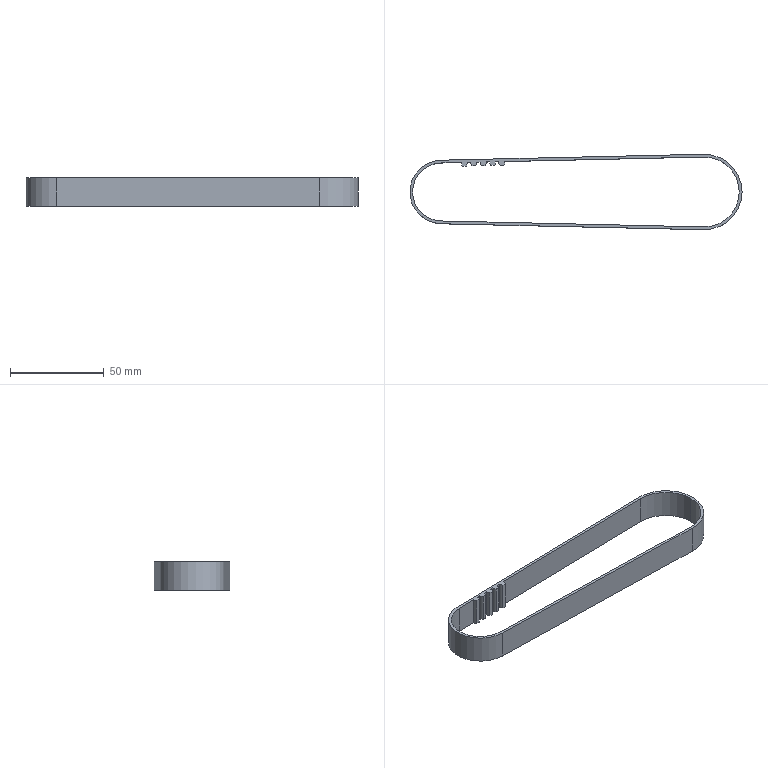Part | SolidWorks | features BaseBody 1 | 1 solid | 37 faces | box 177.014 x 40.237 x 15 mm | volume 9222 mm3 | cylinder 21 | plane 16 | commonest cylinder face diameters 6.5 x15 37.237 x2 40.237 x2 30.871 x1 33.871 x1
STEP:
#1=CARTESIAN_POINT('',(139.502,-20.113,-7.5));
#2=VERTEX_POINT('',#1);
#3=CARTESIAN_POINT('',(160.079,0.,-7.5));
#4=VERTEX_POINT('',#3);
#5=CARTESIAN_POINT('',(139.96,0.,-7.5));
#6=DIRECTION('',(0.,0.,1.));
#7=DIRECTION('',(1.,0.,0.));
#8=AXIS2_PLACEMENT_3D('',#5,#6,#7);
#9=CIRCLE('',#8,20.119);
#10=EDGE_CURVE('',#2,#4,#9,.T.);
#11=ORIENTED_EDGE('',*,*,#10,.T.);
#12=CARTESIAN_POINT('',(160.079,0.,7.5));
#13=VERTEX_POINT('',#12);
#14=CARTESIAN_POINT('',(160.079,0.,7.5));
#15=DIRECTION('',(0.,0.,1.));
#16=VECTOR('',#15,1000.);
#17=LINE('',#14,#16);
#18=EDGE_CURVE('',#4,#13,#17,.T.);
#19=ORIENTED_EDGE('',*,*,#18,.T.);
#20=CARTESIAN_POINT('',(139.502,-20.113,7.5));
#21=VERTEX_POINT('',#20);
#22=CARTESIAN_POINT('',(139.96,0.,7.5));
#23=DIRECTION('',(0.,0.,-1.));
#24=DIRECTION('',(1.,0.,0.));
#25=AXIS2_PLACEMENT_3D('',#22,#23,#24);
#26=CIRCLE('',#25,20.119);
#27=EDGE_CURVE('',#13,#21,#26,.T.);
#28=ORIENTED_EDGE('',*,*,#27,.T.);
#29=CARTESIAN_POINT('',(139.502,-20.113,7.5));
#30=DIRECTION('',(0.,0.,-1.));
#31=VECTOR('',#30,1000.);
#32=LINE('',#29,#31);
#33=EDGE_CURVE('',#21,#2,#32,.T.);
#34=ORIENTED_EDGE('',*,*,#33,.T.);
#35=EDGE_LOOP('',(#11,#19,#28,#34));
#36=FACE_OUTER_BOUND('',#35,.T.);
#37=CARTESIAN_POINT('',(139.96,0.,7.5));
#38=DIRECTION('',(0.,0.,1.));
#39=DIRECTION('',(1.,0.,0.));
#40=AXIS2_PLACEMENT_3D('',#37,#38,#39);
#41=CYLINDRICAL_SURFACE('',#40,20.119);
#42=ADVANCED_FACE('',(#36),#41,.T.);
#43=CARTESIAN_POINT('',(33.188,14.284,-7.5));
#44=VERTEX_POINT('',#43);
#45=CARTESIAN_POINT('',(33.766,16.134,-7.5));
#46=VERTEX_POINT('',#45);
#47=CARTESIAN_POINT('',(30.516,16.134,-7.5));
#48=DIRECTION('',(0.,0.,1.));
#49=DIRECTION('',(1.,0.,0.));
#50=AXIS2_PLACEMENT_3D('',#47,#48,#49);
#51=CIRCLE('',#50,3.25);
#52=EDGE_CURVE('',#44,#46,#51,.T.);
#53=ORIENTED_EDGE('',*,*,#52,.T.);
#54=CARTESIAN_POINT('',(33.766,16.134,7.5));
#55=VERTEX_POINT('',#54);
#56=CARTESIAN_POINT('',(33.766,16.134,7.5));
#57=DIRECTION('',(0.,0.,1.));
#58=VECTOR('',#57,1000.);
#59=LINE('',#56,#58);
#60=EDGE_CURVE('',#46,#55,#59,.T.);
#61=ORIENTED_EDGE('',*,*,#60,.T.);
#62=CARTESIAN_POINT('',(33.188,14.284,7.5));
#63=VERTEX_POINT('',#62);
#64=CARTESIAN_POINT('',(30.516,16.134,7.5));
#65=DIRECTION('',(0.,0.,1.));
#66=DIRECTION('',(1.,0.,0.));
#67=AXIS2_PLACEMENT_3D('',#64,#65,#66);
#68=CIRCLE('',#67,3.25);
#69=EDGE_CURVE('',#63,#55,#68,.T.);
#70=ORIENTED_EDGE('',*,*,#69,.F.);
#71=CARTESIAN_POINT('',(33.188,14.284,7.5));
#72=DIRECTION('',(0.,0.,-1.));
#73=VECTOR('',#72,1000.);
#74=LINE('',#71,#73);
#75=EDGE_CURVE('',#63,#44,#74,.T.);
#76=ORIENTED_EDGE('',*,*,#75,.T.);
#77=EDGE_LOOP('',(#53,#61,#70,#76));
#78=FACE_OUTER_BOUND('',#77,.T.);
#79=CARTESIAN_POINT('',(30.516,16.134,7.5));
#80=DIRECTION('',(0.,0.,1.));
#81=DIRECTION('',(1.,0.,0.));
#82=AXIS2_PLACEMENT_3D('',#79,#80,#81);
#83=CYLINDRICAL_SURFACE('',#82,3.25);
#84=ADVANCED_FACE('',(#78),#83,.T.);
#85=CARTESIAN_POINT('',(28.19,14.17,-7.5));
#86=VERTEX_POINT('',#85);
#87=CARTESIAN_POINT('',(28.767,16.02,-7.5));
#88=VERTEX_POINT('',#87);
#89=CARTESIAN_POINT('',(25.517,16.02,-7.5));
#90=DIRECTION('',(0.,0.,1.));
#91=DIRECTION('',(1.,0.,0.));
#92=AXIS2_PLACEMENT_3D('',#89,#90,#91);
#93=CIRCLE('',#92,3.25);
#94=EDGE_CURVE('',#86,#88,#93,.T.);
#95=ORIENTED_EDGE('',*,*,#94,.T.);
#96=CARTESIAN_POINT('',(28.767,16.02,7.5));
#97=VERTEX_POINT('',#96);
#98=CARTESIAN_POINT('',(28.767,16.02,7.5));
#99=DIRECTION('',(0.,0.,1.));
#100=VECTOR('',#99,1000.);
#101=LINE('',#98,#100);
#102=EDGE_CURVE('',#88,#97,#101,.T.);
#103=ORIENTED_EDGE('',*,*,#102,.T.);
#104=CARTESIAN_POINT('',(28.19,14.17,7.5));
#105=VERTEX_POINT('',#104);
#106=CARTESIAN_POINT('',(25.517,16.02,7.5));
#107=DIRECTION('',(0.,0.,1.));
#108=DIRECTION('',(1.,0.,0.));
#109=AXIS2_PLACEMENT_3D('',#106,#107,#108);
#110=CIRCLE('',#109,3.25);
#111=EDGE_CURVE('',#105,#97,#110,.T.);
#112=ORIENTED_EDGE('',*,*,#111,.F.);
#113=CARTESIAN_POINT('',(28.19,14.17,7.5));
#114=DIRECTION('',(0.,0.,-1.));
#115=VECTOR('',#114,1000.);
#116=LINE('',#113,#115);
#117=EDGE_CURVE('',#105,#86,#116,.T.);
#118=ORIENTED_EDGE('',*,*,#117,.T.);
#119=EDGE_LOOP('',(#95,#103,#112,#118));
#120=FACE_OUTER_BOUND('',#119,.T.);
#121=CARTESIAN_POINT('',(25.517,16.02,7.5));
#122=DIRECTION('',(0.,0.,1.));
#123=DIRECTION('',(1.,0.,0.));
#124=AXIS2_PLACEMENT_3D('',#121,#122,#123);
#125=CYLINDRICAL_SURFACE('',#124,3.25);
#126=ADVANCED_FACE('',(#120),#125,.T.);
#127=CARTESIAN_POINT('',(23.191,14.057,-7.5));
#128=VERTEX_POINT('',#127);
#129=CARTESIAN_POINT('',(23.769,15.906,-7.5));
#130=VERTEX_POINT('',#129);
#131=CARTESIAN_POINT('',(20.519,15.906,-7.5));
#132=DIRECTION('',(0.,0.,1.));
#133=DIRECTION('',(1.,0.,0.));
#134=AXIS2_PLACEMENT_3D('',#131,#132,#133);
#135=CIRCLE('',#134,3.25);
#136=EDGE_CURVE('',#128,#130,#135,.T.);
#137=ORIENTED_EDGE('',*,*,#136,.T.);
#138=CARTESIAN_POINT('',(23.769,15.906,7.5));
#139=VERTEX_POINT('',#138);
#140=CARTESIAN_POINT('',(23.769,15.906,7.5));
#141=DIRECTION('',(0.,0.,1.));
#142=VECTOR('',#141,1000.);
#143=LINE('',#140,#142);
#144=EDGE_CURVE('',#130,#139,#143,.T.);
#145=ORIENTED_EDGE('',*,*,#144,.T.);
#146=CARTESIAN_POINT('',(23.191,14.057,7.5));
#147=VERTEX_POINT('',#146);
#148=CARTESIAN_POINT('',(20.519,15.906,7.5));
#149=DIRECTION('',(0.,0.,1.));
#150=DIRECTION('',(1.,0.,0.));
#151=AXIS2_PLACEMENT_3D('',#148,#149,#150);
#152=CIRCLE('',#151,3.25);
#153=EDGE_CURVE('',#147,#139,#152,.T.);
#154=ORIENTED_EDGE('',*,*,#153,.F.);
#155=CARTESIAN_POINT('',(23.191,14.057,7.5));
#156=DIRECTION('',(0.,0.,-1.));
#157=VECTOR('',#156,1000.);
#158=LINE('',#155,#157);
#159=EDGE_CURVE('',#147,#128,#158,.T.);
#160=ORIENTED_EDGE('',*,*,#159,.T.);
#161=EDGE_LOOP('',(#137,#145,#154,#160));
#162=FACE_OUTER_BOUND('',#161,.T.);
#163=CARTESIAN_POINT('',(20.519,15.906,7.5));
#164=DIRECTION('',(0.,0.,1.));
#165=DIRECTION('',(1.,0.,0.));
#166=AXIS2_PLACEMENT_3D('',#163,#164,#165);
#167=CYLINDRICAL_SURFACE('',#166,3.25);
#168=ADVANCED_FACE('',(#162),#167,.T.);
#169=CARTESIAN_POINT('',(18.192,13.943,-7.5));
#170=VERTEX_POINT('',#169);
#171=CARTESIAN_POINT('',(18.77,15.793,-7.5));
#172=VERTEX_POINT('',#171);
#173=CARTESIAN_POINT('',(15.52,15.793,-7.5));
#174=DIRECTION('',(0.,0.,1.));
#175=DIRECTION('',(1.,0.,0.));
#176=AXIS2_PLACEMENT_3D('',#173,#174,#175);
#177=CIRCLE('',#176,3.25);
#178=EDGE_CURVE('',#170,#172,#177,.T.);
#179=ORIENTED_EDGE('',*,*,#178,.T.);
#180=CARTESIAN_POINT('',(18.77,15.793,7.5));
#181=VERTEX_POINT('',#180);
#182=CARTESIAN_POINT('',(18.77,15.793,7.5));
#183=DIRECTION('',(0.,0.,1.));
#184=VECTOR('',#183,1000.);
#185=LINE('',#182,#184);
#186=EDGE_CURVE('',#172,#181,#185,.T.);
#187=ORIENTED_EDGE('',*,*,#186,.T.);
#188=CARTESIAN_POINT('',(18.192,13.943,7.5));
#189=VERTEX_POINT('',#188);
#190=CARTESIAN_POINT('',(15.52,15.793,7.5));
#191=DIRECTION('',(0.,0.,1.));
#192=DIRECTION('',(1.,0.,0.));
#193=AXIS2_PLACEMENT_3D('',#190,#191,#192);
#194=CIRCLE('',#193,3.25);
#195=EDGE_CURVE('',#189,#181,#194,.T.);
#196=ORIENTED_EDGE('',*,*,#195,.F.);
#197=CARTESIAN_POINT('',(18.192,13.943,7.5));
#198=DIRECTION('',(0.,0.,-1.));
#199=VECTOR('',#198,1000.);
#200=LINE('',#197,#199);
#201=EDGE_CURVE('',#189,#170,#200,.T.);
#202=ORIENTED_EDGE('',*,*,#201,.T.);
#203=EDGE_LOOP('',(#179,#187,#196,#202));
#204=FACE_OUTER_BOUND('',#203,.T.);
#205=CARTESIAN_POINT('',(15.52,15.793,7.5));
#206=DIRECTION('',(0.,0.,1.));
#207=DIRECTION('',(1.,0.,0.));
#208=AXIS2_PLACEMENT_3D('',#205,#206,#207);
#209=CYLINDRICAL_SURFACE('',#208,3.25);
#210=ADVANCED_FACE('',(#204),#209,.T.);
#211=CARTESIAN_POINT('',(13.193,13.829,-7.5));
#212=VERTEX_POINT('',#211);
#213=CARTESIAN_POINT('',(13.771,15.679,-7.5));
#214=VERTEX_POINT('',#213);
#215=CARTESIAN_POINT('',(10.521,15.679,-7.5));
#216=DIRECTION('',(0.,0.,1.));
#217=DIRECTION('',(1.,0.,0.));
#218=AXIS2_PLACEMENT_3D('',#215,#216,#217);
#219=CIRCLE('',#218,3.25);
#220=EDGE_CURVE('',#212,#214,#219,.T.);
#221=ORIENTED_EDGE('',*,*,#220,.T.);
#222=CARTESIAN_POINT('',(13.771,15.679,7.5));
#223=VERTEX_POINT('',#222);
#224=CARTESIAN_POINT('',(13.771,15.679,7.5));
#225=DIRECTION('',(0.,0.,1.));
#226=VECTOR('',#225,1000.);
#227=LINE('',#224,#226);
#228=EDGE_CURVE('',#214,#223,#227,.T.);
#229=ORIENTED_EDGE('',*,*,#228,.T.);
#230=CARTESIAN_POINT('',(13.193,13.829,7.5));
#231=VERTEX_POINT('',#230);
#232=CARTESIAN_POINT('',(10.521,15.679,7.5));
#233=DIRECTION('',(0.,0.,1.));
#234=DIRECTION('',(1.,0.,0.));
#235=AXIS2_PLACEMENT_3D('',#232,#233,#234);
#236=CIRCLE('',#235,3.25);
#237=EDGE_CURVE('',#231,#223,#236,.T.);
#238=ORIENTED_EDGE('',*,*,#237,.F.);
#239=CARTESIAN_POINT('',(13.193,13.829,7.5));
#240=DIRECTION('',(0.,0.,-1.));
#241=VECTOR('',#240,1000.);
#242=LINE('',#239,#241);
#243=EDGE_CURVE('',#231,#212,#242,.T.);
#244=ORIENTED_EDGE('',*,*,#243,.T.);
#245=EDGE_LOOP('',(#221,#229,#238,#244));
#246=FACE_OUTER_BOUND('',#245,.T.);
#247=CARTESIAN_POINT('',(10.521,15.679,7.5));
#248=DIRECTION('',(0.,0.,1.));
#249=DIRECTION('',(1.,0.,0.));
#250=AXIS2_PLACEMENT_3D('',#247,#248,#249);
#251=CYLINDRICAL_SURFACE('',#250,3.25);
#252=ADVANCED_FACE('',(#246),#251,.T.);
#253=CARTESIAN_POINT('',(139.537,18.614,-7.5));
#254=VERTEX_POINT('',#253);
#255=CARTESIAN_POINT('',(158.579,0.,-7.5));
#256=VERTEX_POINT('',#255);
#257=CARTESIAN_POINT('',(139.96,0.,-7.5));
#258=DIRECTION('',(0.,0.,-1.));
#259=DIRECTION('',(1.,0.,0.));
#260=AXIS2_PLACEMENT_3D('',#257,#258,#259);
#261=CIRCLE('',#260,18.619);
#262=EDGE_CURVE('',#254,#256,#261,.T.);
#263=ORIENTED_EDGE('',*,*,#262,.T.);
#264=CARTESIAN_POINT('',(158.579,0.,7.5));
#265=VERTEX_POINT('',#264);
#266=CARTESIAN_POINT('',(158.579,0.,7.5));
#267=DIRECTION('',(0.,0.,1.));
#268=VECTOR('',#267,1000.);
#269=LINE('',#266,#268);
#270=EDGE_CURVE('',#256,#265,#269,.T.);
#271=ORIENTED_EDGE('',*,*,#270,.T.);
#272=CARTESIAN_POINT('',(139.537,18.614,7.5));
#273=VERTEX_POINT('',#272);
#274=CARTESIAN_POINT('',(139.96,0.,7.5));
#275=DIRECTION('',(0.,0.,-1.));
#276=DIRECTION('',(1.,0.,0.));
#277=AXIS2_PLACEMENT_3D('',#274,#275,#276);
#278=CIRCLE('',#277,18.619);
#279=EDGE_CURVE('',#273,#265,#278,.T.);
#280=ORIENTED_EDGE('',*,*,#279,.F.);
#281=CARTESIAN_POINT('',(139.537,18.614,7.5));
#282=DIRECTION('',(0.,0.,1.));
#283=VECTOR('',#282,1000.);
#284=LINE('',#281,#283);
#285=EDGE_CURVE('',#254,#273,#284,.T.);
#286=ORIENTED_EDGE('',*,*,#285,.F.);
#287=EDGE_LOOP('',(#263,#271,#280,#286));
#288=FACE_OUTER_BOUND('',#287,.T.);
#289=CARTESIAN_POINT('',(139.96,0.,7.5));
#290=DIRECTION('',(0.,0.,1.));
#291=DIRECTION('',(1.,0.,0.));
#292=AXIS2_PLACEMENT_3D('',#289,#290,#291);
#293=CYLINDRICAL_SURFACE('',#292,18.619);
#294=ADVANCED_FACE('',(#288),#293,.F.);
#295=CARTESIAN_POINT('',(-0.3852,16.931,7.5));
#296=VERTEX_POINT('',#295);
#297=CARTESIAN_POINT('',(139.502,20.113,7.5));
#298=VERTEX_POINT('',#297);
#299=CARTESIAN_POINT('',(34.606,17.727,7.5));
#300=DIRECTION('',(0.9997,0.02274,0.));
#301=VECTOR('',#300,1000.);
#302=LINE('',#299,#301);
#303=EDGE_CURVE('',#296,#298,#302,.T.);
#304=ORIENTED_EDGE('',*,*,#303,.T.);
#305=CARTESIAN_POINT('',(139.502,20.113,-7.5));
#306=VERTEX_POINT('',#305);
#307=CARTESIAN_POINT('',(139.502,20.113,7.5));
#308=DIRECTION('',(0.,0.,-1.));
#309=VECTOR('',#308,1000.);
#310=LINE('',#307,#309);
#311=EDGE_CURVE('',#298,#306,#310,.T.);
#312=ORIENTED_EDGE('',*,*,#311,.T.);
#313=CARTESIAN_POINT('',(-0.3852,16.931,-7.5));
#314=VERTEX_POINT('',#313);
#315=CARTESIAN_POINT('',(34.606,17.727,-7.5));
#316=DIRECTION('',(-0.9997,-0.02274,0.));
#317=VECTOR('',#316,1000.);
#318=LINE('',#315,#317);
#319=EDGE_CURVE('',#306,#314,#318,.T.);
#320=ORIENTED_EDGE('',*,*,#319,.T.);
#321=CARTESIAN_POINT('',(-0.3852,16.931,7.5));
#322=DIRECTION('',(0.,0.,1.));
#323=VECTOR('',#322,1000.);
#324=LINE('',#321,#323);
#325=EDGE_CURVE('',#314,#296,#324,.T.);
#326=ORIENTED_EDGE('',*,*,#325,.T.);
#327=EDGE_LOOP('',(#304,#312,#320,#326));
#328=FACE_OUTER_BOUND('',#327,.T.);
#329=CARTESIAN_POINT('',(34.606,17.727,7.5));
#330=DIRECTION('',(-0.02274,0.9997,0.));
#331=DIRECTION('',(-0.9997,-0.02274,0.));
#332=AXIS2_PLACEMENT_3D('',#329,#330,#331);
#333=PLANE('',#332);
#334=ADVANCED_FACE('',(#328),#333,.T.);
#335=ORIENTED_EDGE('',*,*,#18,.F.);
#336=CARTESIAN_POINT('',(139.96,0.,-7.5));
#337=DIRECTION('',(0.,0.,1.));
#338=DIRECTION('',(1.,0.,0.));
#339=AXIS2_PLACEMENT_3D('',#336,#337,#338);
#340=CIRCLE('',#339,20.119);
#341=EDGE_CURVE('',#4,#306,#340,.T.);
#342=ORIENTED_EDGE('',*,*,#341,.T.);
#343=ORIENTED_EDGE('',*,*,#311,.F.);
#344=CARTESIAN_POINT('',(139.96,0.,7.5));
#345=DIRECTION('',(0.,0.,-1.));
#346=DIRECTION('',(1.,0.,0.));
#347=AXIS2_PLACEMENT_3D('',#344,#345,#346);
#348=CIRCLE('',#347,20.119);
#349=EDGE_CURVE('',#298,#13,#348,.T.);
#350=ORIENTED_EDGE('',*,*,#349,.T.);
#351=EDGE_LOOP('',(#335,#342,#343,#350));
#352=FACE_OUTER_BOUND('',#351,.T.);
#353=CARTESIAN_POINT('',(139.96,0.,7.5));
#354=DIRECTION('',(0.,0.,1.));
#355=DIRECTION('',(1.,0.,0.));
#356=AXIS2_PLACEMENT_3D('',#353,#354,#355);
#357=CYLINDRICAL_SURFACE('',#356,20.119);
#358=ADVANCED_FACE('',(#352),#357,.T.);
#359=CARTESIAN_POINT('',(31.18,14.238,7.5));
#360=VERTEX_POINT('',#359);
#361=CARTESIAN_POINT('',(31.18,14.238,7.5));
#362=DIRECTION('',(0.9997,0.02274,0.));
#363=VECTOR('',#362,1000.);
#364=LINE('',#361,#363);
#365=EDGE_CURVE('',#360,#63,#364,.T.);
#366=ORIENTED_EDGE('',*,*,#365,.T.);
#367=ORIENTED_EDGE('',*,*,#69,.T.);
#368=CARTESIAN_POINT('',(33.765,16.208,7.5));
#369=VERTEX_POINT('',#368);
#370=CARTESIAN_POINT('',(30.516,16.134,7.5));
#371=DIRECTION('',(0.,0.,1.));
#372=DIRECTION('',(1.,0.,0.));
#373=AXIS2_PLACEMENT_3D('',#370,#371,#372);
#374=CIRCLE('',#373,3.25);
#375=EDGE_CURVE('',#55,#369,#374,.T.);
#376=ORIENTED_EDGE('',*,*,#375,.T.);
#377=CARTESIAN_POINT('',(33.765,16.208,7.5));
#378=DIRECTION('',(0.9997,0.02274,0.));
#379=VECTOR('',#378,1000.);
#380=LINE('',#377,#379);
#381=EDGE_CURVE('',#369,#273,#380,.T.);
#382=ORIENTED_EDGE('',*,*,#381,.T.);
#383=ORIENTED_EDGE('',*,*,#279,.T.);
#384=CARTESIAN_POINT('',(139.537,-18.614,7.5));
#385=VERTEX_POINT('',#384);
#386=CARTESIAN_POINT('',(139.96,0.,7.5));
#387=DIRECTION('',(0.,0.,-1.));
#388=DIRECTION('',(1.,0.,0.));
#389=AXIS2_PLACEMENT_3D('',#386,#387,#388);
#390=CIRCLE('',#389,18.619);
#391=EDGE_CURVE('',#265,#385,#390,.T.);
#392=ORIENTED_EDGE('',*,*,#391,.T.);
#393=CARTESIAN_POINT('',(-0.351,-15.432,7.5));
#394=VERTEX_POINT('',#393);
#395=CARTESIAN_POINT('',(139.537,-18.614,7.5));
#396=DIRECTION('',(-0.9997,0.02274,0.));
#397=VECTOR('',#396,1000.);
#398=LINE('',#395,#397);
#399=EDGE_CURVE('',#385,#394,#398,.T.);
#400=ORIENTED_EDGE('',*,*,#399,.T.);
#401=CARTESIAN_POINT('',(-0.351,15.432,7.5));
#402=VERTEX_POINT('',#401);
#403=CARTESIAN_POINT('',(0.,0.,7.5));
#404=DIRECTION('',(0.,0.,-1.));
#405=DIRECTION('',(1.,0.,0.));
#406=AXIS2_PLACEMENT_3D('',#403,#404,#405);
#407=CIRCLE('',#406,15.435);
#408=EDGE_CURVE('',#394,#402,#407,.T.);
#409=ORIENTED_EDGE('',*,*,#408,.T.);
#410=CARTESIAN_POINT('',(10.521,15.679,7.5));
#411=VERTEX_POINT('',#410);
#412=CARTESIAN_POINT('',(-0.351,15.432,7.5));
#413=DIRECTION('',(0.9997,0.02274,0.));
#414=VECTOR('',#413,1000.);
#415=LINE('',#412,#414);
#416=EDGE_CURVE('',#402,#411,#415,.T.);
#417=ORIENTED_EDGE('',*,*,#416,.T.);
#418=CARTESIAN_POINT('',(11.185,13.783,7.5));
#419=VERTEX_POINT('',#418);
#420=CARTESIAN_POINT('',(13.77,15.753,7.5));
#421=DIRECTION('',(0.,0.,1.));
#422=DIRECTION('',(1.,0.,0.));
#423=AXIS2_PLACEMENT_3D('',#420,#421,#422);
#424=CIRCLE('',#423,3.25);
#425=EDGE_CURVE('',#411,#419,#424,.T.);
#426=ORIENTED_EDGE('',*,*,#425,.T.);
#427=CARTESIAN_POINT('',(11.185,13.783,7.5));
#428=DIRECTION('',(0.9997,0.02274,0.));
#429=VECTOR('',#428,1000.);
#430=LINE('',#427,#429);
#431=EDGE_CURVE('',#419,#231,#430,.T.);
#432=ORIENTED_EDGE('',*,*,#431,.T.);
#433=ORIENTED_EDGE('',*,*,#237,.T.);
#434=CARTESIAN_POINT('',(13.77,15.753,7.5));
#435=VERTEX_POINT('',#434);
#436=CARTESIAN_POINT('',(10.521,15.679,7.5));
#437=DIRECTION('',(0.,0.,1.));
#438=DIRECTION('',(1.,0.,0.));
#439=AXIS2_PLACEMENT_3D('',#436,#437,#438);
#440=CIRCLE('',#439,3.25);
#441=EDGE_CURVE('',#223,#435,#440,.T.);
#442=ORIENTED_EDGE('',*,*,#441,.T.);
#443=CARTESIAN_POINT('',(15.52,15.793,7.5));
#444=VERTEX_POINT('',#443);
#445=CARTESIAN_POINT('',(13.77,15.753,7.5));
#446=DIRECTION('',(0.9997,0.02274,0.));
#447=VECTOR('',#446,1000.);
#448=LINE('',#445,#447);
#449=EDGE_CURVE('',#435,#444,#448,.T.);
#450=ORIENTED_EDGE('',*,*,#449,.T.);
#451=CARTESIAN_POINT('',(16.184,13.897,7.5));
#452=VERTEX_POINT('',#451);
#453=CARTESIAN_POINT('',(18.769,15.866,7.5));
#454=DIRECTION('',(0.,0.,1.));
#455=DIRECTION('',(1.,0.,0.));
#456=AXIS2_PLACEMENT_3D('',#453,#454,#455);
#457=CIRCLE('',#456,3.25);
#458=EDGE_CURVE('',#444,#452,#457,.T.);
#459=ORIENTED_EDGE('',*,*,#458,.T.);
#460=CARTESIAN_POINT('',(16.184,13.897,7.5));
#461=DIRECTION('',(0.9997,0.02274,0.));
#462=VECTOR('',#461,1000.);
#463=LINE('',#460,#462);
#464=EDGE_CURVE('',#452,#189,#463,.T.);
#465=ORIENTED_EDGE('',*,*,#464,.T.);
#466=ORIENTED_EDGE('',*,*,#195,.T.);
#467=CARTESIAN_POINT('',(18.769,15.866,7.5));
#468=VERTEX_POINT('',#467);
#469=CARTESIAN_POINT('',(15.52,15.793,7.5));
#470=DIRECTION('',(0.,0.,1.));
#471=DIRECTION('',(1.,0.,0.));
#472=AXIS2_PLACEMENT_3D('',#469,#470,#471);
#473=CIRCLE('',#472,3.25);
#474=EDGE_CURVE('',#181,#468,#473,.T.);
#475=ORIENTED_EDGE('',*,*,#474,.T.);
#476=CARTESIAN_POINT('',(20.519,15.906,7.5));
#477=VERTEX_POINT('',#476);
#478=CARTESIAN_POINT('',(18.769,15.866,7.5));
#479=DIRECTION('',(0.9997,0.02274,0.));
#480=VECTOR('',#479,1000.);
#481=LINE('',#478,#480);
#482=EDGE_CURVE('',#468,#477,#481,.T.);
#483=ORIENTED_EDGE('',*,*,#482,.T.);
#484=CARTESIAN_POINT('',(21.182,14.011,7.5));
#485=VERTEX_POINT('',#484);
#486=CARTESIAN_POINT('',(23.768,15.98,7.5));
#487=DIRECTION('',(0.,0.,1.));
#488=DIRECTION('',(1.,0.,0.));
#489=AXIS2_PLACEMENT_3D('',#486,#487,#488);
#490=CIRCLE('',#489,3.25);
#491=EDGE_CURVE('',#477,#485,#490,.T.);
#492=ORIENTED_EDGE('',*,*,#491,.T.);
#493=CARTESIAN_POINT('',(21.182,14.011,7.5));
#494=DIRECTION('',(0.9997,0.02274,0.));
#495=VECTOR('',#494,1000.);
#496=LINE('',#493,#495);
#497=EDGE_CURVE('',#485,#147,#496,.T.);
#498=ORIENTED_EDGE('',*,*,#497,.T.);
#499=ORIENTED_EDGE('',*,*,#153,.T.);
#500=CARTESIAN_POINT('',(23.768,15.98,7.5));
#501=VERTEX_POINT('',#500);
#502=CARTESIAN_POINT('',(20.519,15.906,7.5));
#503=DIRECTION('',(0.,0.,1.));
#504=DIRECTION('',(1.,0.,0.));
#505=AXIS2_PLACEMENT_3D('',#502,#503,#504);
#506=CIRCLE('',#505,3.25);
#507=EDGE_CURVE('',#139,#501,#506,.T.);
#508=ORIENTED_EDGE('',*,*,#507,.T.);
#509=CARTESIAN_POINT('',(25.517,16.02,7.5));
#510=VERTEX_POINT('',#509);
#511=CARTESIAN_POINT('',(23.768,15.98,7.5));
#512=DIRECTION('',(0.9997,0.02274,0.));
#513=VECTOR('',#512,1000.);
#514=LINE('',#511,#513);
#515=EDGE_CURVE('',#501,#510,#514,.T.);
#516=ORIENTED_EDGE('',*,*,#515,.T.);
#517=CARTESIAN_POINT('',(26.181,14.125,7.5));
#518=VERTEX_POINT('',#517);
#519=CARTESIAN_POINT('',(28.766,16.094,7.5));
#520=DIRECTION('',(0.,0.,1.));
#521=DIRECTION('',(1.,0.,0.));
#522=AXIS2_PLACEMENT_3D('',#519,#520,#521);
#523=CIRCLE('',#522,3.25);
#524=EDGE_CURVE('',#510,#518,#523,.T.);
#525=ORIENTED_EDGE('',*,*,#524,.T.);
#526=CARTESIAN_POINT('',(26.181,14.125,7.5));
#527=DIRECTION('',(0.9997,0.02274,0.));
#528=VECTOR('',#527,1000.);
#529=LINE('',#526,#528);
#530=EDGE_CURVE('',#518,#105,#529,.T.);
#531=ORIENTED_EDGE('',*,*,#530,.T.);
#532=ORIENTED_EDGE('',*,*,#111,.T.);
#533=CARTESIAN_POINT('',(28.766,16.094,7.5));
#534=VERTEX_POINT('',#533);
#535=CARTESIAN_POINT('',(25.517,16.02,7.5));
#536=DIRECTION('',(0.,0.,1.));
#537=DIRECTION('',(1.,0.,0.));
#538=AXIS2_PLACEMENT_3D('',#535,#536,#537);
#539=CIRCLE('',#538,3.25);
#540=EDGE_CURVE('',#97,#534,#539,.T.);
#541=ORIENTED_EDGE('',*,*,#540,.T.);
#542=CARTESIAN_POINT('',(30.516,16.134,7.5));
#543=VERTEX_POINT('',#542);
#544=CARTESIAN_POINT('',(28.766,16.094,7.5));
#545=DIRECTION('',(0.9997,0.02274,0.));
#546=VECTOR('',#545,1000.);
#547=LINE('',#544,#546);
#548=EDGE_CURVE('',#534,#543,#547,.T.);
#549=ORIENTED_EDGE('',*,*,#548,.T.);
#550=CARTESIAN_POINT('',(33.765,16.208,7.5));
#551=DIRECTION('',(0.,0.,1.));
#552=DIRECTION('',(1.,0.,0.));
#553=AXIS2_PLACEMENT_3D('',#550,#551,#552);
#554=CIRCLE('',#553,3.25);
#555=EDGE_CURVE('',#543,#360,#554,.T.);
#556=ORIENTED_EDGE('',*,*,#555,.T.);
#557=EDGE_LOOP('',(#366,#367,#376,#382,#383,#392,#400,#409,#417,#426,#432,#433,#442,#450,#459,#465,#466,#475,#483,#492,#498,#499,#508,#516,#525,#531,#532,#541,#549,#556));
#558=FACE_BOUND('',#557,.T.);
#559=CARTESIAN_POINT('',(-0.3852,-16.931,7.5));
#560=VERTEX_POINT('',#559);
#561=CARTESIAN_POINT('',(-0.3852,-16.931,7.5));
#562=DIRECTION('',(0.9997,-0.02274,0.));
#563=VECTOR('',#562,1000.);
#564=LINE('',#561,#563);
#565=EDGE_CURVE('',#560,#21,#564,.T.);
#566=ORIENTED_EDGE('',*,*,#565,.T.);
#567=ORIENTED_EDGE('',*,*,#27,.F.);
#568=ORIENTED_EDGE('',*,*,#349,.F.);
#569=ORIENTED_EDGE('',*,*,#303,.F.);
#570=CARTESIAN_POINT('',(0.,0.,7.5));
#571=DIRECTION('',(0.,0.,1.));
#572=DIRECTION('',(1.,0.,0.));
#573=AXIS2_PLACEMENT_3D('',#570,#571,#572);
#574=CIRCLE('',#573,16.935);
#575=EDGE_CURVE('',#296,#560,#574,.T.);
#576=ORIENTED_EDGE('',*,*,#575,.T.);
#577=EDGE_LOOP('',(#566,#567,#568,#569,#576));
#578=FACE_OUTER_BOUND('',#577,.T.);
#579=CARTESIAN_POINT('',(0.,0.,7.5));
#580=DIRECTION('',(0.,0.,1.));
#581=DIRECTION('',(1.,0.,0.));
#582=AXIS2_PLACEMENT_3D('',#579,#580,#581);
#583=PLANE('',#582);
#584=ADVANCED_FACE('',(#558,#578),#583,.T.);
#585=ORIENTED_EDGE('',*,*,#575,.F.);
#586=ORIENTED_EDGE('',*,*,#325,.F.);
#587=CARTESIAN_POINT('',(-0.3852,-16.931,-7.5));
#588=VERTEX_POINT('',#587);
#589=CARTESIAN_POINT('',(0.,0.,-7.5));
#590=DIRECTION('',(0.,0.,1.));
#591=DIRECTION('',(1.,0.,0.));
#592=AXIS2_PLACEMENT_3D('',#589,#590,#591);
#593=CIRCLE('',#592,16.935);
#594=EDGE_CURVE('',#314,#588,#593,.T.);
#595=ORIENTED_EDGE('',*,*,#594,.T.);
#596=CARTESIAN_POINT('',(-0.3852,-16.931,7.5));
#597=DIRECTION('',(0.,0.,1.));
#598=VECTOR('',#597,1000.);
#599=LINE('',#596,#598);
#600=EDGE_CURVE('',#588,#560,#599,.T.);
#601=ORIENTED_EDGE('',*,*,#600,.T.);
#602=EDGE_LOOP('',(#585,#586,#595,#601));
#603=FACE_OUTER_BOUND('',#602,.T.);
#604=CARTESIAN_POINT('',(0.,0.,7.5));
#605=DIRECTION('',(0.,0.,1.));
#606=DIRECTION('',(1.,0.,0.));
#607=AXIS2_PLACEMENT_3D('',#604,#605,#606);
#608=CYLINDRICAL_SURFACE('',#607,16.935);
#609=ADVANCED_FACE('',(#603),#608,.T.);
#610=ORIENTED_EDGE('',*,*,#10,.F.);
#611=CARTESIAN_POINT('',(-0.3852,-16.931,-7.5));
#612=DIRECTION('',(0.9997,-0.02274,0.));
#613=VECTOR('',#612,1000.);
#614=LINE('',#611,#613);
#615=EDGE_CURVE('',#588,#2,#614,.T.);
#616=ORIENTED_EDGE('',*,*,#615,.F.);
#617=ORIENTED_EDGE('',*,*,#594,.F.);
#618=ORIENTED_EDGE('',*,*,#319,.F.);
#619=ORIENTED_EDGE('',*,*,#341,.F.);
#620=EDGE_LOOP('',(#610,#616,#617,#618,#619));
#621=FACE_OUTER_BOUND('',#620,.T.);
#622=ORIENTED_EDGE('',*,*,#52,.F.);
#623=CARTESIAN_POINT('',(31.18,14.238,-7.5));
#624=VERTEX_POINT('',#623);
#625=CARTESIAN_POINT('',(31.18,14.238,-7.5));
#626=DIRECTION('',(0.9997,0.02274,0.));
#627=VECTOR('',#626,1000.);
#628=LINE('',#625,#627);
#629=EDGE_CURVE('',#624,#44,#628,.T.);
#630=ORIENTED_EDGE('',*,*,#629,.F.);
#631=CARTESIAN_POINT('',(30.516,16.134,-7.5));
#632=VERTEX_POINT('',#631);
#633=CARTESIAN_POINT('',(33.765,16.208,-7.5));
#634=DIRECTION('',(0.,0.,1.));
#635=DIRECTION('',(1.,0.,0.));
#636=AXIS2_PLACEMENT_3D('',#633,#634,#635);
#637=CIRCLE('',#636,3.25);
#638=EDGE_CURVE('',#632,#624,#637,.T.);
#639=ORIENTED_EDGE('',*,*,#638,.F.);
#640=CARTESIAN_POINT('',(28.766,16.094,-7.5));
#641=VERTEX_POINT('',#640);
#642=CARTESIAN_POINT('',(28.766,16.094,-7.5));
#643=DIRECTION('',(0.9997,0.02274,0.));
#644=VECTOR('',#643,1000.);
#645=LINE('',#642,#644);
#646=EDGE_CURVE('',#641,#632,#645,.T.);
#647=ORIENTED_EDGE('',*,*,#646,.F.);
#648=CARTESIAN_POINT('',(25.517,16.02,-7.5));
#649=DIRECTION('',(0.,0.,1.));
#650=DIRECTION('',(1.,0.,0.));
#651=AXIS2_PLACEMENT_3D('',#648,#649,#650);
#652=CIRCLE('',#651,3.25);
#653=EDGE_CURVE('',#88,#641,#652,.T.);
#654=ORIENTED_EDGE('',*,*,#653,.F.);
#655=ORIENTED_EDGE('',*,*,#94,.F.);
#656=CARTESIAN_POINT('',(26.181,14.125,-7.5));
#657=VERTEX_POINT('',#656);
#658=CARTESIAN_POINT('',(26.181,14.125,-7.5));
#659=DIRECTION('',(0.9997,0.02274,0.));
#660=VECTOR('',#659,1000.);
#661=LINE('',#658,#660);
#662=EDGE_CURVE('',#657,#86,#661,.T.);
#663=ORIENTED_EDGE('',*,*,#662,.F.);
#664=CARTESIAN_POINT('',(25.517,16.02,-7.5));
#665=VERTEX_POINT('',#664);
#666=CARTESIAN_POINT('',(28.766,16.094,-7.5));
#667=DIRECTION('',(0.,0.,1.));
#668=DIRECTION('',(1.,0.,0.));
#669=AXIS2_PLACEMENT_3D('',#666,#667,#668);
#670=CIRCLE('',#669,3.25);
#671=EDGE_CURVE('',#665,#657,#670,.T.);
#672=ORIENTED_EDGE('',*,*,#671,.F.);
#673=CARTESIAN_POINT('',(23.768,15.98,-7.5));
#674=VERTEX_POINT('',#673);
#675=CARTESIAN_POINT('',(23.768,15.98,-7.5));
#676=DIRECTION('',(0.9997,0.02274,0.));
#677=VECTOR('',#676,1000.);
#678=LINE('',#675,#677);
#679=EDGE_CURVE('',#674,#665,#678,.T.);
#680=ORIENTED_EDGE('',*,*,#679,.F.);
#681=CARTESIAN_POINT('',(20.519,15.906,-7.5));
#682=DIRECTION('',(0.,0.,1.));
#683=DIRECTION('',(1.,0.,0.));
#684=AXIS2_PLACEMENT_3D('',#681,#682,#683);
#685=CIRCLE('',#684,3.25);
#686=EDGE_CURVE('',#130,#674,#685,.T.);
#687=ORIENTED_EDGE('',*,*,#686,.F.);
#688=ORIENTED_EDGE('',*,*,#136,.F.);
#689=CARTESIAN_POINT('',(21.182,14.011,-7.5));
#690=VERTEX_POINT('',#689);
#691=CARTESIAN_POINT('',(21.182,14.011,-7.5));
#692=DIRECTION('',(0.9997,0.02274,0.));
#693=VECTOR('',#692,1000.);
#694=LINE('',#691,#693);
#695=EDGE_CURVE('',#690,#128,#694,.T.);
#696=ORIENTED_EDGE('',*,*,#695,.F.);
#697=CARTESIAN_POINT('',(20.519,15.906,-7.5));
#698=VERTEX_POINT('',#697);
#699=CARTESIAN_POINT('',(23.768,15.98,-7.5));
#700=DIRECTION('',(0.,0.,1.));
#701=DIRECTION('',(1.,0.,0.));
#702=AXIS2_PLACEMENT_3D('',#699,#700,#701);
#703=CIRCLE('',#702,3.25);
#704=EDGE_CURVE('',#698,#690,#703,.T.);
#705=ORIENTED_EDGE('',*,*,#704,.F.);
#706=CARTESIAN_POINT('',(18.769,15.866,-7.5));
#707=VERTEX_POINT('',#706);
#708=CARTESIAN_POINT('',(18.769,15.866,-7.5));
#709=DIRECTION('',(0.9997,0.02274,0.));
#710=VECTOR('',#709,1000.);
#711=LINE('',#708,#710);
#712=EDGE_CURVE('',#707,#698,#711,.T.);
#713=ORIENTED_EDGE('',*,*,#712,.F.);
#714=CARTESIAN_POINT('',(15.52,15.793,-7.5));
#715=DIRECTION('',(0.,0.,1.));
#716=DIRECTION('',(1.,0.,0.));
#717=AXIS2_PLACEMENT_3D('',#714,#715,#716);
#718=CIRCLE('',#717,3.25);
#719=EDGE_CURVE('',#172,#707,#718,.T.);
#720=ORIENTED_EDGE('',*,*,#719,.F.);
#721=ORIENTED_EDGE('',*,*,#178,.F.);
#722=CARTESIAN_POINT('',(16.184,13.897,-7.5));
#723=VERTEX_POINT('',#722);
#724=CARTESIAN_POINT('',(16.184,13.897,-7.5));
#725=DIRECTION('',(0.9997,0.02274,0.));
#726=VECTOR('',#725,1000.);
#727=LINE('',#724,#726);
#728=EDGE_CURVE('',#723,#170,#727,.T.);
#729=ORIENTED_EDGE('',*,*,#728,.F.);
#730=CARTESIAN_POINT('',(15.52,15.793,-7.5));
#731=VERTEX_POINT('',#730);
#732=CARTESIAN_POINT('',(18.769,15.866,-7.5));
#733=DIRECTION('',(0.,0.,1.));
#734=DIRECTION('',(1.,0.,0.));
#735=AXIS2_PLACEMENT_3D('',#732,#733,#734);
#736=CIRCLE('',#735,3.25);
#737=EDGE_CURVE('',#731,#723,#736,.T.);
#738=ORIENTED_EDGE('',*,*,#737,.F.);
#739=CARTESIAN_POINT('',(13.77,15.753,-7.5));
#740=VERTEX_POINT('',#739);
#741=CARTESIAN_POINT('',(13.77,15.753,-7.5));
#742=DIRECTION('',(0.9997,0.02274,0.));
#743=VECTOR('',#742,1000.);
#744=LINE('',#741,#743);
#745=EDGE_CURVE('',#740,#731,#744,.T.);
#746=ORIENTED_EDGE('',*,*,#745,.F.);
#747=CARTESIAN_POINT('',(10.521,15.679,-7.5));
#748=DIRECTION('',(0.,0.,1.));
#749=DIRECTION('',(1.,0.,0.));
#750=AXIS2_PLACEMENT_3D('',#747,#748,#749);
#751=CIRCLE('',#750,3.25);
#752=EDGE_CURVE('',#214,#740,#751,.T.);
#753=ORIENTED_EDGE('',*,*,#752,.F.);
#754=ORIENTED_EDGE('',*,*,#220,.F.);
#755=CARTESIAN_POINT('',(11.185,13.783,-7.5));
#756=VERTEX_POINT('',#755);
#757=CARTESIAN_POINT('',(11.185,13.783,-7.5));
#758=DIRECTION('',(0.9997,0.02274,0.));
#759=VECTOR('',#758,1000.);
#760=LINE('',#757,#759);
#761=EDGE_CURVE('',#756,#212,#760,.T.);
#762=ORIENTED_EDGE('',*,*,#761,.F.);
#763=CARTESIAN_POINT('',(10.521,15.679,-7.5));
#764=VERTEX_POINT('',#763);
#765=CARTESIAN_POINT('',(13.77,15.753,-7.5));
#766=DIRECTION('',(0.,0.,1.));
#767=DIRECTION('',(1.,0.,0.));
#768=AXIS2_PLACEMENT_3D('',#765,#766,#767);
#769=CIRCLE('',#768,3.25);
#770=EDGE_CURVE('',#764,#756,#769,.T.);
#771=ORIENTED_EDGE('',*,*,#770,.F.);
#772=CARTESIAN_POINT('',(-0.351,15.432,-7.5));
#773=VERTEX_POINT('',#772);
#774=CARTESIAN_POINT('',(-0.351,15.432,-7.5));
#775=DIRECTION('',(0.9997,0.02274,0.));
#776=VECTOR('',#775,1000.);
#777=LINE('',#774,#776);
#778=EDGE_CURVE('',#773,#764,#777,.T.);
#779=ORIENTED_EDGE('',*,*,#778,.F.);
#780=CARTESIAN_POINT('',(-0.351,-15.432,-7.5));
#781=VERTEX_POINT('',#780);
#782=CARTESIAN_POINT('',(0.,0.,-7.5));
#783=DIRECTION('',(0.,0.,-1.));
#784=DIRECTION('',(1.,0.,0.));
#785=AXIS2_PLACEMENT_3D('',#782,#783,#784);
#786=CIRCLE('',#785,15.435);
#787=EDGE_CURVE('',#781,#773,#786,.T.);
#788=ORIENTED_EDGE('',*,*,#787,.F.);
#789=CARTESIAN_POINT('',(139.537,-18.614,-7.5));
#790=VERTEX_POINT('',#789);
#791=CARTESIAN_POINT('',(139.537,-18.614,-7.5));
#792=DIRECTION('',(-0.9997,0.02274,0.));
#793=VECTOR('',#792,1000.);
#794=LINE('',#791,#793);
#795=EDGE_CURVE('',#790,#781,#794,.T.);
#796=ORIENTED_EDGE('',*,*,#795,.F.);
#797=CARTESIAN_POINT('',(139.96,0.,-7.5));
#798=DIRECTION('',(0.,0.,-1.));
#799=DIRECTION('',(1.,0.,0.));
#800=AXIS2_PLACEMENT_3D('',#797,#798,#799);
#801=CIRCLE('',#800,18.619);
#802=EDGE_CURVE('',#256,#790,#801,.T.);
#803=ORIENTED_EDGE('',*,*,#802,.F.);
#804=ORIENTED_EDGE('',*,*,#262,.F.);
#805=CARTESIAN_POINT('',(33.765,16.208,-7.5));
#806=VERTEX_POINT('',#805);
#807=CARTESIAN_POINT('',(33.765,16.208,-7.5));
#808=DIRECTION('',(0.9997,0.02274,0.));
#809=VECTOR('',#808,1000.);
#810=LINE('',#807,#809);
#811=EDGE_CURVE('',#806,#254,#810,.T.);
#812=ORIENTED_EDGE('',*,*,#811,.F.);
#813=CARTESIAN_POINT('',(30.516,16.134,-7.5));
#814=DIRECTION('',(0.,0.,1.));
#815=DIRECTION('',(1.,0.,0.));
#816=AXIS2_PLACEMENT_3D('',#813,#814,#815);
#817=CIRCLE('',#816,3.25);
#818=EDGE_CURVE('',#46,#806,#817,.T.);
#819=ORIENTED_EDGE('',*,*,#818,.F.);
#820=EDGE_LOOP('',(#622,#630,#639,#647,#654,#655,#663,#672,#680,#687,#688,#696,#705,#713,#720,#721,#729,#738,#746,#753,#754,#762,#771,#779,#788,#796,#803,#804,#812,#819));
#821=FACE_BOUND('',#820,.T.);
#822=CARTESIAN_POINT('',(0.,0.,-7.5));
#823=DIRECTION('',(0.,0.,1.));
#824=DIRECTION('',(1.,0.,0.));
#825=AXIS2_PLACEMENT_3D('',#822,#823,#824);
#826=PLANE('',#825);
#827=ADVANCED_FACE('',(#621,#821),#826,.F.);
#828=ORIENTED_EDGE('',*,*,#60,.F.);
#829=ORIENTED_EDGE('',*,*,#818,.T.);
#830=CARTESIAN_POINT('',(33.765,16.208,7.5));
#831=DIRECTION('',(0.,0.,1.));
#832=VECTOR('',#831,1000.);
#833=LINE('',#830,#832);
#834=EDGE_CURVE('',#806,#369,#833,.T.);
#835=ORIENTED_EDGE('',*,*,#834,.T.);
#836=ORIENTED_EDGE('',*,*,#375,.F.);
#837=EDGE_LOOP('',(#828,#829,#835,#836));
#838=FACE_OUTER_BOUND('',#837,.T.);
#839=CARTESIAN_POINT('',(30.516,16.134,7.5));
#840=DIRECTION('',(0.,0.,1.));
#841=DIRECTION('',(1.,0.,0.));
#842=AXIS2_PLACEMENT_3D('',#839,#840,#841);
#843=CYLINDRICAL_SURFACE('',#842,3.25);
#844=ADVANCED_FACE('',(#838),#843,.T.);
#845=ORIENTED_EDGE('',*,*,#365,.F.);
#846=CARTESIAN_POINT('',(31.18,14.238,7.5));
#847=DIRECTION('',(0.,0.,-1.));
#848=VECTOR('',#847,1000.);
#849=LINE('',#846,#848);
#850=EDGE_CURVE('',#360,#624,#849,.T.);
#851=ORIENTED_EDGE('',*,*,#850,.T.);
#852=ORIENTED_EDGE('',*,*,#629,.T.);
#853=ORIENTED_EDGE('',*,*,#75,.F.);
#854=EDGE_LOOP('',(#845,#851,#852,#853));
#855=FACE_OUTER_BOUND('',#854,.T.);
#856=CARTESIAN_POINT('',(31.18,14.238,7.5));
#857=DIRECTION('',(0.02274,-0.9997,0.));
#858=DIRECTION('',(0.9997,0.02274,0.));
#859=AXIS2_PLACEMENT_3D('',#856,#857,#858);
#860=PLANE('',#859);
#861=ADVANCED_FACE('',(#855),#860,.T.);
#862=ORIENTED_EDGE('',*,*,#555,.F.);
#863=CARTESIAN_POINT('',(30.516,16.134,7.5));
#864=DIRECTION('',(0.,0.,-1.));
#865=VECTOR('',#864,1000.);
#866=LINE('',#863,#865);
#867=EDGE_CURVE('',#543,#632,#866,.T.);
#868=ORIENTED_EDGE('',*,*,#867,.T.);
#869=ORIENTED_EDGE('',*,*,#638,.T.);
#870=ORIENTED_EDGE('',*,*,#850,.F.);
#871=EDGE_LOOP('',(#862,#868,#869,#870));
#872=FACE_OUTER_BOUND('',#871,.T.);
#873=CARTESIAN_POINT('',(33.765,16.208,7.5));
#874=DIRECTION('',(0.,0.,1.));
#875=DIRECTION('',(1.,0.,0.));
#876=AXIS2_PLACEMENT_3D('',#873,#874,#875);
#877=CYLINDRICAL_SURFACE('',#876,3.25);
#878=ADVANCED_FACE('',(#872),#877,.T.);
#879=ORIENTED_EDGE('',*,*,#548,.F.);
#880=CARTESIAN_POINT('',(28.766,16.094,7.5));
#881=DIRECTION('',(0.,0.,-1.));
#882=VECTOR('',#881,1000.);
#883=LINE('',#880,#882);
#884=EDGE_CURVE('',#534,#641,#883,.T.);
#885=ORIENTED_EDGE('',*,*,#884,.T.);
#886=ORIENTED_EDGE('',*,*,#646,.T.);
#887=ORIENTED_EDGE('',*,*,#867,.F.);
#888=EDGE_LOOP('',(#879,#885,#886,#887));
#889=FACE_OUTER_BOUND('',#888,.T.);
#890=CARTESIAN_POINT('',(28.766,16.094,7.5));
#891=DIRECTION('',(0.02274,-0.9997,0.));
#892=DIRECTION('',(0.9997,0.02274,0.));
#893=AXIS2_PLACEMENT_3D('',#890,#891,#892);
#894=PLANE('',#893);
#895=ADVANCED_FACE('',(#889),#894,.T.);
#896=ORIENTED_EDGE('',*,*,#102,.F.);
#897=ORIENTED_EDGE('',*,*,#653,.T.);
#898=ORIENTED_EDGE('',*,*,#884,.F.);
#899=ORIENTED_EDGE('',*,*,#540,.F.);
#900=EDGE_LOOP('',(#896,#897,#898,#899));
#901=FACE_OUTER_BOUND('',#900,.T.);
#902=CARTESIAN_POINT('',(25.517,16.02,7.5));
#903=DIRECTION('',(0.,0.,1.));
#904=DIRECTION('',(1.,0.,0.));
#905=AXIS2_PLACEMENT_3D('',#902,#903,#904);
#906=CYLINDRICAL_SURFACE('',#905,3.25);
#907=ADVANCED_FACE('',(#901),#906,.T.);
#908=ORIENTED_EDGE('',*,*,#530,.F.);
#909=CARTESIAN_POINT('',(26.181,14.125,7.5));
#910=DIRECTION('',(0.,0.,-1.));
#911=VECTOR('',#910,1000.);
#912=LINE('',#909,#911);
#913=EDGE_CURVE('',#518,#657,#912,.T.);
#914=ORIENTED_EDGE('',*,*,#913,.T.);
#915=ORIENTED_EDGE('',*,*,#662,.T.);
#916=ORIENTED_EDGE('',*,*,#117,.F.);
#917=EDGE_LOOP('',(#908,#914,#915,#916));
#918=FACE_OUTER_BOUND('',#917,.T.);
#919=CARTESIAN_POINT('',(26.181,14.125,7.5));
#920=DIRECTION('',(0.02274,-0.9997,0.));
#921=DIRECTION('',(0.9997,0.02274,0.));
#922=AXIS2_PLACEMENT_3D('',#919,#920,#921);
#923=PLANE('',#922);
#924=ADVANCED_FACE('',(#918),#923,.T.);
#925=ORIENTED_EDGE('',*,*,#524,.F.);
#926=CARTESIAN_POINT('',(25.517,16.02,7.5));
#927=DIRECTION('',(0.,0.,-1.));
#928=VECTOR('',#927,1000.);
#929=LINE('',#926,#928);
#930=EDGE_CURVE('',#510,#665,#929,.T.);
#931=ORIENTED_EDGE('',*,*,#930,.T.);
#932=ORIENTED_EDGE('',*,*,#671,.T.);
#933=ORIENTED_EDGE('',*,*,#913,.F.);
#934=EDGE_LOOP('',(#925,#931,#932,#933));
#935=FACE_OUTER_BOUND('',#934,.T.);
#936=CARTESIAN_POINT('',(28.766,16.094,7.5));
#937=DIRECTION('',(0.,0.,1.));
#938=DIRECTION('',(1.,0.,0.));
#939=AXIS2_PLACEMENT_3D('',#936,#937,#938);
#940=CYLINDRICAL_SURFACE('',#939,3.25);
#941=ADVANCED_FACE('',(#935),#940,.T.);
#942=ORIENTED_EDGE('',*,*,#515,.F.);
#943=CARTESIAN_POINT('',(23.768,15.98,7.5));
#944=DIRECTION('',(0.,0.,-1.));
#945=VECTOR('',#944,1000.);
#946=LINE('',#943,#945);
#947=EDGE_CURVE('',#501,#674,#946,.T.);
#948=ORIENTED_EDGE('',*,*,#947,.T.);
#949=ORIENTED_EDGE('',*,*,#679,.T.);
#950=ORIENTED_EDGE('',*,*,#930,.F.);
#951=EDGE_LOOP('',(#942,#948,#949,#950));
#952=FACE_OUTER_BOUND('',#951,.T.);
#953=CARTESIAN_POINT('',(23.768,15.98,7.5));
#954=DIRECTION('',(0.02274,-0.9997,0.));
#955=DIRECTION('',(0.9997,0.02274,0.));
#956=AXIS2_PLACEMENT_3D('',#953,#954,#955);
#957=PLANE('',#956);
#958=ADVANCED_FACE('',(#952),#957,.T.);
#959=ORIENTED_EDGE('',*,*,#144,.F.);
#960=ORIENTED_EDGE('',*,*,#686,.T.);
#961=ORIENTED_EDGE('',*,*,#947,.F.);
#962=ORIENTED_EDGE('',*,*,#507,.F.);
#963=EDGE_LOOP('',(#959,#960,#961,#962));
#964=FACE_OUTER_BOUND('',#963,.T.);
#965=CARTESIAN_POINT('',(20.519,15.906,7.5));
#966=DIRECTION('',(0.,0.,1.));
#967=DIRECTION('',(1.,0.,0.));
#968=AXIS2_PLACEMENT_3D('',#965,#966,#967);
#969=CYLINDRICAL_SURFACE('',#968,3.25);
#970=ADVANCED_FACE('',(#964),#969,.T.);
#971=ORIENTED_EDGE('',*,*,#497,.F.);
#972=CARTESIAN_POINT('',(21.182,14.011,7.5));
#973=DIRECTION('',(0.,0.,-1.));
#974=VECTOR('',#973,1000.);
#975=LINE('',#972,#974);
#976=EDGE_CURVE('',#485,#690,#975,.T.);
#977=ORIENTED_EDGE('',*,*,#976,.T.);
#978=ORIENTED_EDGE('',*,*,#695,.T.);
#979=ORIENTED_EDGE('',*,*,#159,.F.);
#980=EDGE_LOOP('',(#971,#977,#978,#979));
#981=FACE_OUTER_BOUND('',#980,.T.);
#982=CARTESIAN_POINT('',(21.182,14.011,7.5));
#983=DIRECTION('',(0.02274,-0.9997,0.));
#984=DIRECTION('',(0.9997,0.02274,0.));
#985=AXIS2_PLACEMENT_3D('',#982,#983,#984);
#986=PLANE('',#985);
#987=ADVANCED_FACE('',(#981),#986,.T.);
#988=ORIENTED_EDGE('',*,*,#491,.F.);
#989=CARTESIAN_POINT('',(20.519,15.906,7.5));
#990=DIRECTION('',(0.,0.,-1.));
#991=VECTOR('',#990,1000.);
#992=LINE('',#989,#991);
#993=EDGE_CURVE('',#477,#698,#992,.T.);
#994=ORIENTED_EDGE('',*,*,#993,.T.);
#995=ORIENTED_EDGE('',*,*,#704,.T.);
#996=ORIENTED_EDGE('',*,*,#976,.F.);
#997=EDGE_LOOP('',(#988,#994,#995,#996));
#998=FACE_OUTER_BOUND('',#997,.T.);
#999=CARTESIAN_POINT('',(23.768,15.98,7.5));
#1000=DIRECTION('',(0.,0.,1.));
#1001=DIRECTION('',(1.,0.,0.));
#1002=AXIS2_PLACEMENT_3D('',#999,#1000,#1001);
#1003=CYLINDRICAL_SURFACE('',#1002,3.25);
#1004=ADVANCED_FACE('',(#998),#1003,.T.);
#1005=ORIENTED_EDGE('',*,*,#482,.F.);
#1006=CARTESIAN_POINT('',(18.769,15.866,7.5));
#1007=DIRECTION('',(0.,0.,-1.));
#1008=VECTOR('',#1007,1000.);
#1009=LINE('',#1006,#1008);
#1010=EDGE_CURVE('',#468,#707,#1009,.T.);
#1011=ORIENTED_EDGE('',*,*,#1010,.T.);
#1012=ORIENTED_EDGE('',*,*,#712,.T.);
#1013=ORIENTED_EDGE('',*,*,#993,.F.);
#1014=EDGE_LOOP('',(#1005,#1011,#1012,#1013));
#1015=FACE_OUTER_BOUND('',#1014,.T.);
#1016=CARTESIAN_POINT('',(18.769,15.866,7.5));
#1017=DIRECTION('',(0.02274,-0.9997,0.));
#1018=DIRECTION('',(0.9997,0.02274,0.));
#1019=AXIS2_PLACEMENT_3D('',#1016,#1017,#1018);
#1020=PLANE('',#1019);
#1021=ADVANCED_FACE('',(#1015),#1020,.T.);
#1022=ORIENTED_EDGE('',*,*,#186,.F.);
#1023=ORIENTED_EDGE('',*,*,#719,.T.);
#1024=ORIENTED_EDGE('',*,*,#1010,.F.);
#1025=ORIENTED_EDGE('',*,*,#474,.F.);
#1026=EDGE_LOOP('',(#1022,#1023,#1024,#1025));
#1027=FACE_OUTER_BOUND('',#1026,.T.);
#1028=CARTESIAN_POINT('',(15.52,15.793,7.5));
#1029=DIRECTION('',(0.,0.,1.));
#1030=DIRECTION('',(1.,0.,0.));
#1031=AXIS2_PLACEMENT_3D('',#1028,#1029,#1030);
#1032=CYLINDRICAL_SURFACE('',#1031,3.25);
#1033=ADVANCED_FACE('',(#1027),#1032,.T.);
#1034=ORIENTED_EDGE('',*,*,#464,.F.);
#1035=CARTESIAN_POINT('',(16.184,13.897,7.5));
#1036=DIRECTION('',(0.,0.,-1.));
#1037=VECTOR('',#1036,1000.);
#1038=LINE('',#1035,#1037);
#1039=EDGE_CURVE('',#452,#723,#1038,.T.);
#1040=ORIENTED_EDGE('',*,*,#1039,.T.);
#1041=ORIENTED_EDGE('',*,*,#728,.T.);
#1042=ORIENTED_EDGE('',*,*,#201,.F.);
#1043=EDGE_LOOP('',(#1034,#1040,#1041,#1042));
#1044=FACE_OUTER_BOUND('',#1043,.T.);
#1045=CARTESIAN_POINT('',(16.184,13.897,7.5));
#1046=DIRECTION('',(0.02274,-0.9997,0.));
#1047=DIRECTION('',(0.9997,0.02274,0.));
#1048=AXIS2_PLACEMENT_3D('',#1045,#1046,#1047);
#1049=PLANE('',#1048);
#1050=ADVANCED_FACE('',(#1044),#1049,.T.);
#1051=ORIENTED_EDGE('',*,*,#458,.F.);
#1052=CARTESIAN_POINT('',(15.52,15.793,7.5));
#1053=DIRECTION('',(0.,0.,-1.));
#1054=VECTOR('',#1053,1000.);
#1055=LINE('',#1052,#1054);
#1056=EDGE_CURVE('',#444,#731,#1055,.T.);
#1057=ORIENTED_EDGE('',*,*,#1056,.T.);
#1058=ORIENTED_EDGE('',*,*,#737,.T.);
#1059=ORIENTED_EDGE('',*,*,#1039,.F.);
#1060=EDGE_LOOP('',(#1051,#1057,#1058,#1059));
#1061=FACE_OUTER_BOUND('',#1060,.T.);
#1062=CARTESIAN_POINT('',(18.769,15.866,7.5));
#1063=DIRECTION('',(0.,0.,1.));
#1064=DIRECTION('',(1.,0.,0.));
#1065=AXIS2_PLACEMENT_3D('',#1062,#1063,#1064);
#1066=CYLINDRICAL_SURFACE('',#1065,3.25);
#1067=ADVANCED_FACE('',(#1061),#1066,.T.);
#1068=ORIENTED_EDGE('',*,*,#449,.F.);
#1069=CARTESIAN_POINT('',(13.77,15.753,7.5));
#1070=DIRECTION('',(0.,0.,-1.));
#1071=VECTOR('',#1070,1000.);
#1072=LINE('',#1069,#1071);
#1073=EDGE_CURVE('',#435,#740,#1072,.T.);
#1074=ORIENTED_EDGE('',*,*,#1073,.T.);
#1075=ORIENTED_EDGE('',*,*,#745,.T.);
#1076=ORIENTED_EDGE('',*,*,#1056,.F.);
#1077=EDGE_LOOP('',(#1068,#1074,#1075,#1076));
#1078=FACE_OUTER_BOUND('',#1077,.T.);
#1079=CARTESIAN_POINT('',(13.77,15.753,7.5));
#1080=DIRECTION('',(0.02274,-0.9997,0.));
#1081=DIRECTION('',(0.9997,0.02274,0.));
#1082=AXIS2_PLACEMENT_3D('',#1079,#1080,#1081);
#1083=PLANE('',#1082);
#1084=ADVANCED_FACE('',(#1078),#1083,.T.);
#1085=ORIENTED_EDGE('',*,*,#228,.F.);
#1086=ORIENTED_EDGE('',*,*,#752,.T.);
#1087=ORIENTED_EDGE('',*,*,#1073,.F.);
#1088=ORIENTED_EDGE('',*,*,#441,.F.);
#1089=EDGE_LOOP('',(#1085,#1086,#1087,#1088));
#1090=FACE_OUTER_BOUND('',#1089,.T.);
#1091=CARTESIAN_POINT('',(10.521,15.679,7.5));
#1092=DIRECTION('',(0.,0.,1.));
#1093=DIRECTION('',(1.,0.,0.));
#1094=AXIS2_PLACEMENT_3D('',#1091,#1092,#1093);
#1095=CYLINDRICAL_SURFACE('',#1094,3.25);
#1096=ADVANCED_FACE('',(#1090),#1095,.T.);
#1097=ORIENTED_EDGE('',*,*,#431,.F.);
#1098=CARTESIAN_POINT('',(11.185,13.783,7.5));
#1099=DIRECTION('',(0.,0.,-1.));
#1100=VECTOR('',#1099,1000.);
#1101=LINE('',#1098,#1100);
#1102=EDGE_CURVE('',#419,#756,#1101,.T.);
#1103=ORIENTED_EDGE('',*,*,#1102,.T.);
#1104=ORIENTED_EDGE('',*,*,#761,.T.);
#1105=ORIENTED_EDGE('',*,*,#243,.F.);
#1106=EDGE_LOOP('',(#1097,#1103,#1104,#1105));
#1107=FACE_OUTER_BOUND('',#1106,.T.);
#1108=CARTESIAN_POINT('',(11.185,13.783,7.5));
#1109=DIRECTION('',(0.02274,-0.9997,0.));
#1110=DIRECTION('',(0.9997,0.02274,0.));
#1111=AXIS2_PLACEMENT_3D('',#1108,#1109,#1110);
#1112=PLANE('',#1111);
#1113=ADVANCED_FACE('',(#1107),#1112,.T.);
#1114=ORIENTED_EDGE('',*,*,#425,.F.);
#1115=CARTESIAN_POINT('',(10.521,15.679,7.5));
#1116=DIRECTION('',(0.,0.,-1.));
#1117=VECTOR('',#1116,1000.);
#1118=LINE('',#1115,#1117);
#1119=EDGE_CURVE('',#411,#764,#1118,.T.);
#1120=ORIENTED_EDGE('',*,*,#1119,.T.);
#1121=ORIENTED_EDGE('',*,*,#770,.T.);
#1122=ORIENTED_EDGE('',*,*,#1102,.F.);
#1123=EDGE_LOOP('',(#1114,#1120,#1121,#1122));
#1124=FACE_OUTER_BOUND('',#1123,.T.);
#1125=CARTESIAN_POINT('',(13.77,15.753,7.5));
#1126=DIRECTION('',(0.,0.,1.));
#1127=DIRECTION('',(1.,0.,0.));
#1128=AXIS2_PLACEMENT_3D('',#1125,#1126,#1127);
#1129=CYLINDRICAL_SURFACE('',#1128,3.25);
#1130=ADVANCED_FACE('',(#1124),#1129,.T.);
#1131=ORIENTED_EDGE('',*,*,#416,.F.);
#1132=CARTESIAN_POINT('',(-0.351,15.432,7.5));
#1133=DIRECTION('',(0.,0.,-1.));
#1134=VECTOR('',#1133,1000.);
#1135=LINE('',#1132,#1134);
#1136=EDGE_CURVE('',#402,#773,#1135,.T.);
#1137=ORIENTED_EDGE('',*,*,#1136,.T.);
#1138=ORIENTED_EDGE('',*,*,#778,.T.);
#1139=ORIENTED_EDGE('',*,*,#1119,.F.);
#1140=EDGE_LOOP('',(#1131,#1137,#1138,#1139));
#1141=FACE_OUTER_BOUND('',#1140,.T.);
#1142=CARTESIAN_POINT('',(9.646,15.659,7.5));
#1143=DIRECTION('',(0.02274,-0.9997,0.));
#1144=DIRECTION('',(0.9997,0.02274,0.));
#1145=AXIS2_PLACEMENT_3D('',#1142,#1143,#1144);
#1146=PLANE('',#1145);
#1147=ADVANCED_FACE('',(#1141),#1146,.T.);
#1148=ORIENTED_EDGE('',*,*,#1136,.F.);
#1149=ORIENTED_EDGE('',*,*,#408,.F.);
#1150=CARTESIAN_POINT('',(-0.351,-15.432,7.5));
#1151=DIRECTION('',(0.,0.,1.));
#1152=VECTOR('',#1151,1000.);
#1153=LINE('',#1150,#1152);
#1154=EDGE_CURVE('',#781,#394,#1153,.T.);
#1155=ORIENTED_EDGE('',*,*,#1154,.F.);
#1156=ORIENTED_EDGE('',*,*,#787,.T.);
#1157=EDGE_LOOP('',(#1148,#1149,#1155,#1156));
#1158=FACE_OUTER_BOUND('',#1157,.T.);
#1159=CARTESIAN_POINT('',(0.,0.,7.5));
#1160=DIRECTION('',(0.,0.,1.));
#1161=DIRECTION('',(1.,0.,0.));
#1162=AXIS2_PLACEMENT_3D('',#1159,#1160,#1161);
#1163=CYLINDRICAL_SURFACE('',#1162,15.435);
#1164=ADVANCED_FACE('',(#1158),#1163,.F.);
#1165=ORIENTED_EDGE('',*,*,#399,.F.);
#1166=CARTESIAN_POINT('',(139.537,-18.614,7.5));
#1167=DIRECTION('',(0.,0.,-1.));
#1168=VECTOR('',#1167,1000.);
#1169=LINE('',#1166,#1168);
#1170=EDGE_CURVE('',#385,#790,#1169,.T.);
#1171=ORIENTED_EDGE('',*,*,#1170,.T.);
#1172=ORIENTED_EDGE('',*,*,#795,.T.);
#1173=ORIENTED_EDGE('',*,*,#1154,.T.);
#1174=EDGE_LOOP('',(#1165,#1171,#1172,#1173));
#1175=FACE_OUTER_BOUND('',#1174,.T.);
#1176=CARTESIAN_POINT('',(139.537,-18.614,7.5));
#1177=DIRECTION('',(0.02274,0.9997,0.));
#1178=DIRECTION('',(-0.9997,0.02274,0.));
#1179=AXIS2_PLACEMENT_3D('',#1176,#1177,#1178);
#1180=PLANE('',#1179);
#1181=ADVANCED_FACE('',(#1175),#1180,.T.);
#1182=ORIENTED_EDGE('',*,*,#270,.F.);
#1183=ORIENTED_EDGE('',*,*,#802,.T.);
#1184=ORIENTED_EDGE('',*,*,#1170,.F.);
#1185=ORIENTED_EDGE('',*,*,#391,.F.);
#1186=EDGE_LOOP('',(#1182,#1183,#1184,#1185));
#1187=FACE_OUTER_BOUND('',#1186,.T.);
#1188=CARTESIAN_POINT('',(139.96,0.,7.5));
#1189=DIRECTION('',(0.,0.,1.));
#1190=DIRECTION('',(1.,0.,0.));
#1191=AXIS2_PLACEMENT_3D('',#1188,#1189,#1190);
#1192=CYLINDRICAL_SURFACE('',#1191,18.619);
#1193=ADVANCED_FACE('',(#1187),#1192,.F.);
#1194=ORIENTED_EDGE('',*,*,#381,.F.);
#1195=ORIENTED_EDGE('',*,*,#834,.F.);
#1196=ORIENTED_EDGE('',*,*,#811,.T.);
#1197=ORIENTED_EDGE('',*,*,#285,.T.);
#1198=EDGE_LOOP('',(#1194,#1195,#1196,#1197));
#1199=FACE_OUTER_BOUND('',#1198,.T.);
#1200=CARTESIAN_POINT('',(33.765,16.208,7.5));
#1201=DIRECTION('',(0.02274,-0.9997,0.));
#1202=DIRECTION('',(0.9997,0.02274,0.));
#1203=AXIS2_PLACEMENT_3D('',#1200,#1201,#1202);
#1204=PLANE('',#1203);
#1205=ADVANCED_FACE('',(#1199),#1204,.T.);
#1206=ORIENTED_EDGE('',*,*,#565,.F.);
#1207=ORIENTED_EDGE('',*,*,#600,.F.);
#1208=ORIENTED_EDGE('',*,*,#615,.T.);
#1209=ORIENTED_EDGE('',*,*,#33,.F.);
#1210=EDGE_LOOP('',(#1206,#1207,#1208,#1209));
#1211=FACE_OUTER_BOUND('',#1210,.T.);
#1212=CARTESIAN_POINT('',(-0.3852,-16.931,7.5));
#1213=DIRECTION('',(-0.02274,-0.9997,0.));
#1214=DIRECTION('',(0.9997,-0.02274,0.));
#1215=AXIS2_PLACEMENT_3D('',#1212,#1213,#1214);
#1216=PLANE('',#1215);
#1217=ADVANCED_FACE('',(#1211),#1216,.T.);
#1218=CLOSED_SHELL('',(#42,#84,#126,#168,#210,#252,#294,#334,#358,#584,#609,#827,#844,#861,#878,#895,#907,#924,#941,#958,#970,#987,#1004,#1021,#1033,#1050,#1067,#1084,#1096,#1113,#1130,#1147,#1164,#1181,#1193,#1205,#1217));
#1219=MANIFOLD_SOLID_BREP('',#1218);
#1220=CARTESIAN_POINT('',(0.,0.,0.));
#1221=DIRECTION('',(0.,0.,1.));
#1222=DIRECTION('',(1.,0.,0.));
#1223=AXIS2_PLACEMENT_3D('',#1220,#1221,#1222);
#1224=(LENGTH_UNIT()NAMED_UNIT(*)SI_UNIT(.MILLI.,.METRE.));
#1225=UNCERTAINTY_MEASURE_WITH_UNIT(LENGTH_MEASURE(0.00001),#1224,'','');
#1226=(NAMED_UNIT(*)PLANE_ANGLE_UNIT()SI_UNIT($,.RADIAN.));
#1227=(NAMED_UNIT(*)SI_UNIT($,.STERADIAN.)SOLID_ANGLE_UNIT());
#1228=(GEOMETRIC_REPRESENTATION_CONTEXT(3)GLOBAL_UNCERTAINTY_ASSIGNED_CONTEXT((#1225))GLOBAL_UNIT_ASSIGNED_CONTEXT((#1224,#1226,#1227))REPRESENTATION_CONTEXT('',''));
#1229=ADVANCED_BREP_SHAPE_REPRESENTATION('',(#1219,#1223),#1228);